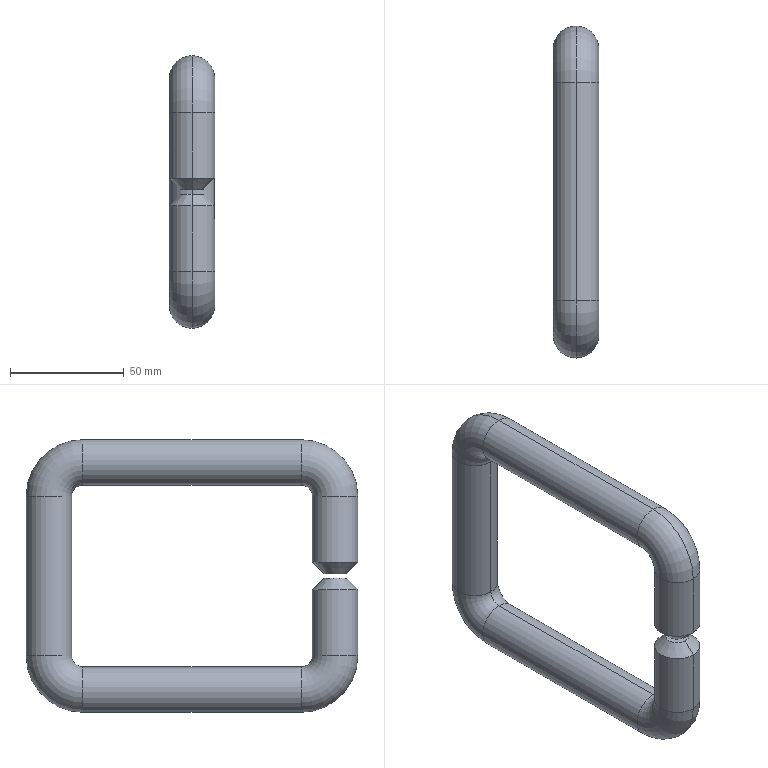Part | SolidWorks | features Chamfer 1, Sweep 1 | 1 solid | 24 faces | box 20 x 146 x 120 mm | volume 131972 mm3 | cylinder 10 | torus 8 | cone 4 | plane 2 | commonest cylinder face diameters 20 x10
STEP:
#1=CARTESIAN_POINT('',(0.,10.,34.));
#2=VERTEX_POINT('',#1);
#3=CARTESIAN_POINT('',(0.,-10.,34.));
#4=VERTEX_POINT('',#3);
#5=CARTESIAN_POINT('',(0.,0.,34.));
#6=DIRECTION('',(0.,0.,1.));
#7=DIRECTION('',(1.,0.,0.));
#8=AXIS2_PLACEMENT_3D('',#5,#6,#7);
#9=CIRCLE('',#8,10.);
#10=EDGE_CURVE('',#2,#4,#9,.T.);
#11=ORIENTED_EDGE('',*,*,#10,.T.);
#12=CARTESIAN_POINT('',(0.,15.,59.));
#13=VERTEX_POINT('',#12);
#14=CARTESIAN_POINT('',(0.,15.,34.));
#15=DIRECTION('',(-1.,0.,0.));
#16=DIRECTION('',(0.,0.,1.));
#17=AXIS2_PLACEMENT_3D('',#14,#15,#16);
#18=CIRCLE('',#17,25.);
#19=EDGE_CURVE('',#4,#13,#18,.T.);
#20=ORIENTED_EDGE('',*,*,#19,.T.);
#21=CARTESIAN_POINT('',(0.,15.,39.));
#22=VERTEX_POINT('',#21);
#23=CARTESIAN_POINT('',(0.,15.,49.));
#24=DIRECTION('',(0.,1.,0.));
#25=DIRECTION('',(1.,0.,0.));
#26=AXIS2_PLACEMENT_3D('',#23,#24,#25);
#27=CIRCLE('',#26,10.);
#28=EDGE_CURVE('',#22,#13,#27,.T.);
#29=ORIENTED_EDGE('',*,*,#28,.F.);
#30=CARTESIAN_POINT('',(0.,15.,34.));
#31=DIRECTION('',(-1.,0.,0.));
#32=DIRECTION('',(0.,0.,1.));
#33=AXIS2_PLACEMENT_3D('',#30,#31,#32);
#34=CIRCLE('',#33,5.);
#35=EDGE_CURVE('',#2,#22,#34,.T.);
#36=ORIENTED_EDGE('',*,*,#35,.F.);
#37=EDGE_LOOP('',(#11,#20,#29,#36));
#38=FACE_OUTER_BOUND('',#37,.T.);
#39=CARTESIAN_POINT('',(0.,15.,34.));
#40=DIRECTION('',(-1.,0.,0.));
#41=DIRECTION('',(0.,0.,1.));
#42=AXIS2_PLACEMENT_3D('',#39,#40,#41);
#43=TOROIDAL_SURFACE('',#42,15.,10.);
#44=ADVANCED_FACE('',(#38),#43,.T.);
#45=CARTESIAN_POINT('',(0.,111.,39.));
#46=VERTEX_POINT('',#45);
#47=CARTESIAN_POINT('',(0.,111.,59.));
#48=VERTEX_POINT('',#47);
#49=CARTESIAN_POINT('',(0.,111.,49.));
#50=DIRECTION('',(0.,1.,0.));
#51=DIRECTION('',(1.,0.,0.));
#52=AXIS2_PLACEMENT_3D('',#49,#50,#51);
#53=CIRCLE('',#52,10.);
#54=EDGE_CURVE('',#46,#48,#53,.T.);
#55=ORIENTED_EDGE('',*,*,#54,.T.);
#56=CARTESIAN_POINT('',(0.,136.,34.));
#57=VERTEX_POINT('',#56);
#58=CARTESIAN_POINT('',(0.,111.,34.));
#59=DIRECTION('',(-1.,0.,0.));
#60=DIRECTION('',(0.,0.,1.));
#61=AXIS2_PLACEMENT_3D('',#58,#59,#60);
#62=CIRCLE('',#61,25.);
#63=EDGE_CURVE('',#48,#57,#62,.T.);
#64=ORIENTED_EDGE('',*,*,#63,.T.);
#65=CARTESIAN_POINT('',(0.,116.,34.));
#66=VERTEX_POINT('',#65);
#67=CARTESIAN_POINT('',(0.,126.,34.));
#68=DIRECTION('',(0.,0.,-1.));
#69=DIRECTION('',(1.,0.,0.));
#70=AXIS2_PLACEMENT_3D('',#67,#68,#69);
#71=CIRCLE('',#70,10.);
#72=EDGE_CURVE('',#66,#57,#71,.T.);
#73=ORIENTED_EDGE('',*,*,#72,.F.);
#74=CARTESIAN_POINT('',(0.,111.,34.));
#75=DIRECTION('',(-1.,0.,0.));
#76=DIRECTION('',(0.,0.,1.));
#77=AXIS2_PLACEMENT_3D('',#74,#75,#76);
#78=CIRCLE('',#77,5.);
#79=EDGE_CURVE('',#46,#66,#78,.T.);
#80=ORIENTED_EDGE('',*,*,#79,.F.);
#81=EDGE_LOOP('',(#55,#64,#73,#80));
#82=FACE_OUTER_BOUND('',#81,.T.);
#83=CARTESIAN_POINT('',(0.,111.,34.));
#84=DIRECTION('',(-1.,0.,0.));
#85=DIRECTION('',(0.,0.,1.));
#86=AXIS2_PLACEMENT_3D('',#83,#84,#85);
#87=TOROIDAL_SURFACE('',#86,15.,10.);
#88=ADVANCED_FACE('',(#82),#87,.T.);
#89=CARTESIAN_POINT('',(0.,116.,-36.));
#90=VERTEX_POINT('',#89);
#91=CARTESIAN_POINT('',(0.,136.,-36.));
#92=VERTEX_POINT('',#91);
#93=CARTESIAN_POINT('',(0.,126.,-36.));
#94=DIRECTION('',(0.,0.,-1.));
#95=DIRECTION('',(1.,0.,0.));
#96=AXIS2_PLACEMENT_3D('',#93,#94,#95);
#97=CIRCLE('',#96,10.);
#98=EDGE_CURVE('',#90,#92,#97,.T.);
#99=ORIENTED_EDGE('',*,*,#98,.T.);
#100=CARTESIAN_POINT('',(0.,111.,-61.));
#101=VERTEX_POINT('',#100);
#102=CARTESIAN_POINT('',(0.,111.,-36.));
#103=DIRECTION('',(-1.,0.,0.));
#104=DIRECTION('',(0.,0.,1.));
#105=AXIS2_PLACEMENT_3D('',#102,#103,#104);
#106=CIRCLE('',#105,25.);
#107=EDGE_CURVE('',#92,#101,#106,.T.);
#108=ORIENTED_EDGE('',*,*,#107,.T.);
#109=CARTESIAN_POINT('',(0.,111.,-41.));
#110=VERTEX_POINT('',#109);
#111=CARTESIAN_POINT('',(0.,111.,-51.));
#112=DIRECTION('',(0.,-1.,0.));
#113=DIRECTION('',(1.,0.,0.));
#114=AXIS2_PLACEMENT_3D('',#111,#112,#113);
#115=CIRCLE('',#114,10.);
#116=EDGE_CURVE('',#110,#101,#115,.T.);
#117=ORIENTED_EDGE('',*,*,#116,.F.);
#118=CARTESIAN_POINT('',(0.,111.,-36.));
#119=DIRECTION('',(-1.,0.,0.));
#120=DIRECTION('',(0.,0.,1.));
#121=AXIS2_PLACEMENT_3D('',#118,#119,#120);
#122=CIRCLE('',#121,5.);
#123=EDGE_CURVE('',#90,#110,#122,.T.);
#124=ORIENTED_EDGE('',*,*,#123,.F.);
#125=EDGE_LOOP('',(#99,#108,#117,#124));
#126=FACE_OUTER_BOUND('',#125,.T.);
#127=CARTESIAN_POINT('',(0.,111.,-36.));
#128=DIRECTION('',(-1.,0.,0.));
#129=DIRECTION('',(0.,0.,1.));
#130=AXIS2_PLACEMENT_3D('',#127,#128,#129);
#131=TOROIDAL_SURFACE('',#130,15.,10.);
#132=ADVANCED_FACE('',(#126),#131,.T.);
#133=CARTESIAN_POINT('',(0.,15.,-41.));
#134=VERTEX_POINT('',#133);
#135=CARTESIAN_POINT('',(0.,15.,-61.));
#136=VERTEX_POINT('',#135);
#137=CARTESIAN_POINT('',(0.,15.,-51.));
#138=DIRECTION('',(0.,-1.,0.));
#139=DIRECTION('',(1.,0.,0.));
#140=AXIS2_PLACEMENT_3D('',#137,#138,#139);
#141=CIRCLE('',#140,10.);
#142=EDGE_CURVE('',#134,#136,#141,.T.);
#143=ORIENTED_EDGE('',*,*,#142,.T.);
#144=CARTESIAN_POINT('',(0.,-10.,-36.));
#145=VERTEX_POINT('',#144);
#146=CARTESIAN_POINT('',(0.,15.,-36.));
#147=DIRECTION('',(-1.,0.,0.));
#148=DIRECTION('',(0.,0.,1.));
#149=AXIS2_PLACEMENT_3D('',#146,#147,#148);
#150=CIRCLE('',#149,25.);
#151=EDGE_CURVE('',#136,#145,#150,.T.);
#152=ORIENTED_EDGE('',*,*,#151,.T.);
#153=CARTESIAN_POINT('',(0.,10.,-36.));
#154=VERTEX_POINT('',#153);
#155=CARTESIAN_POINT('',(0.,0.,-36.));
#156=DIRECTION('',(0.,0.,1.));
#157=DIRECTION('',(1.,0.,0.));
#158=AXIS2_PLACEMENT_3D('',#155,#156,#157);
#159=CIRCLE('',#158,10.);
#160=EDGE_CURVE('',#154,#145,#159,.T.);
#161=ORIENTED_EDGE('',*,*,#160,.F.);
#162=CARTESIAN_POINT('',(0.,15.,-36.));
#163=DIRECTION('',(-1.,0.,0.));
#164=DIRECTION('',(0.,0.,1.));
#165=AXIS2_PLACEMENT_3D('',#162,#163,#164);
#166=CIRCLE('',#165,5.);
#167=EDGE_CURVE('',#134,#154,#166,.T.);
#168=ORIENTED_EDGE('',*,*,#167,.F.);
#169=EDGE_LOOP('',(#143,#152,#161,#168));
#170=FACE_OUTER_BOUND('',#169,.T.);
#171=CARTESIAN_POINT('',(0.,15.,-36.));
#172=DIRECTION('',(-1.,0.,0.));
#173=DIRECTION('',(0.,0.,1.));
#174=AXIS2_PLACEMENT_3D('',#171,#172,#173);
#175=TOROIDAL_SURFACE('',#174,15.,10.);
#176=ADVANCED_FACE('',(#170),#175,.T.);
#177=CARTESIAN_POINT('',(0.,5.,0.));
#178=VERTEX_POINT('',#177);
#179=CARTESIAN_POINT('',(0.,-5.,0.));
#180=VERTEX_POINT('',#179);
#181=CARTESIAN_POINT('',(0.,0.,0.));
#182=DIRECTION('',(0.,0.,-1.));
#183=DIRECTION('',(1.,0.,0.));
#184=AXIS2_PLACEMENT_3D('',#181,#182,#183);
#185=CIRCLE('',#184,5.);
#186=EDGE_CURVE('',#178,#180,#185,.T.);
#187=ORIENTED_EDGE('',*,*,#186,.F.);
#188=CARTESIAN_POINT('',(0.,10.,5.));
#189=VERTEX_POINT('',#188);
#190=CARTESIAN_POINT('',(0.,10.,5.));
#191=DIRECTION('',(0.,0.7071,0.7071));
#192=VECTOR('',#191,1000.);
#193=LINE('',#190,#192);
#194=EDGE_CURVE('',#178,#189,#193,.T.);
#195=ORIENTED_EDGE('',*,*,#194,.T.);
#196=CARTESIAN_POINT('',(0.,-10.,5.));
#197=VERTEX_POINT('',#196);
#198=CARTESIAN_POINT('',(0.,0.,5.));
#199=DIRECTION('',(0.,0.,1.));
#200=DIRECTION('',(0.,-1.,0.));
#201=AXIS2_PLACEMENT_3D('',#198,#199,#200);
#202=CIRCLE('',#201,10.);
#203=EDGE_CURVE('',#197,#189,#202,.T.);
#204=ORIENTED_EDGE('',*,*,#203,.F.);
#205=CARTESIAN_POINT('',(0.,-10.,5.));
#206=DIRECTION('',(0.,-0.7071,0.7071));
#207=VECTOR('',#206,1000.);
#208=LINE('',#205,#207);
#209=EDGE_CURVE('',#180,#197,#208,.T.);
#210=ORIENTED_EDGE('',*,*,#209,.F.);
#211=EDGE_LOOP('',(#187,#195,#204,#210));
#212=FACE_OUTER_BOUND('',#211,.T.);
#213=CARTESIAN_POINT('',(0.,0.,5.));
#214=DIRECTION('',(0.,0.,1.));
#215=DIRECTION('',(0.,-1.,0.));
#216=AXIS2_PLACEMENT_3D('',#213,#214,#215);
#217=CONICAL_SURFACE('',#216,10.,0.7854);
#218=ADVANCED_FACE('',(#212),#217,.T.);
#219=CARTESIAN_POINT('',(0.,-5.,-2.));
#220=VERTEX_POINT('',#219);
#221=CARTESIAN_POINT('',(0.,5.,-2.));
#222=VERTEX_POINT('',#221);
#223=CARTESIAN_POINT('',(0.,0.,-2.));
#224=DIRECTION('',(0.,0.,1.));
#225=DIRECTION('',(0.,-1.,0.));
#226=AXIS2_PLACEMENT_3D('',#223,#224,#225);
#227=CIRCLE('',#226,5.);
#228=EDGE_CURVE('',#220,#222,#227,.T.);
#229=ORIENTED_EDGE('',*,*,#228,.F.);
#230=CARTESIAN_POINT('',(0.,-10.,-7.));
#231=VERTEX_POINT('',#230);
#232=CARTESIAN_POINT('',(0.,-5.,-2.));
#233=DIRECTION('',(0.,-0.7071,-0.7071));
#234=VECTOR('',#233,1000.);
#235=LINE('',#232,#234);
#236=EDGE_CURVE('',#220,#231,#235,.T.);
#237=ORIENTED_EDGE('',*,*,#236,.T.);
#238=CARTESIAN_POINT('',(0.,10.,-7.));
#239=VERTEX_POINT('',#238);
#240=CARTESIAN_POINT('',(0.,0.,-7.));
#241=DIRECTION('',(0.,0.,-1.));
#242=DIRECTION('',(0.,-1.,0.));
#243=AXIS2_PLACEMENT_3D('',#240,#241,#242);
#244=CIRCLE('',#243,10.);
#245=EDGE_CURVE('',#239,#231,#244,.T.);
#246=ORIENTED_EDGE('',*,*,#245,.F.);
#247=CARTESIAN_POINT('',(0.,5.,-2.));
#248=DIRECTION('',(0.,0.7071,-0.7071));
#249=VECTOR('',#248,1000.);
#250=LINE('',#247,#249);
#251=EDGE_CURVE('',#222,#239,#250,.T.);
#252=ORIENTED_EDGE('',*,*,#251,.F.);
#253=EDGE_LOOP('',(#229,#237,#246,#252));
#254=FACE_OUTER_BOUND('',#253,.T.);
#255=CARTESIAN_POINT('',(0.,0.,-2.));
#256=DIRECTION('',(0.,0.,-1.));
#257=DIRECTION('',(0.,1.,0.));
#258=AXIS2_PLACEMENT_3D('',#255,#256,#257);
#259=CONICAL_SURFACE('',#258,5.,0.7854);
#260=ADVANCED_FACE('',(#254),#259,.T.);
#261=CARTESIAN_POINT('',(0.,0.,34.));
#262=DIRECTION('',(0.,0.,1.));
#263=DIRECTION('',(1.,0.,0.));
#264=AXIS2_PLACEMENT_3D('',#261,#262,#263);
#265=CIRCLE('',#264,10.);
#266=EDGE_CURVE('',#4,#2,#265,.T.);
#267=ORIENTED_EDGE('',*,*,#266,.F.);
#268=CARTESIAN_POINT('',(0.,-10.,34.));
#269=DIRECTION('',(0.,0.,-1.));
#270=VECTOR('',#269,1000.);
#271=LINE('',#268,#270);
#272=EDGE_CURVE('',#4,#197,#271,.T.);
#273=ORIENTED_EDGE('',*,*,#272,.T.);
#274=ORIENTED_EDGE('',*,*,#203,.T.);
#275=CARTESIAN_POINT('',(0.,10.,34.));
#276=DIRECTION('',(0.,0.,-1.));
#277=VECTOR('',#276,1000.);
#278=LINE('',#275,#277);
#279=EDGE_CURVE('',#2,#189,#278,.T.);
#280=ORIENTED_EDGE('',*,*,#279,.F.);
#281=EDGE_LOOP('',(#267,#273,#274,#280));
#282=FACE_OUTER_BOUND('',#281,.T.);
#283=CARTESIAN_POINT('',(0.,0.,34.));
#284=DIRECTION('',(0.,0.,-1.));
#285=DIRECTION('',(0.,1.,0.));
#286=AXIS2_PLACEMENT_3D('',#283,#284,#285);
#287=CYLINDRICAL_SURFACE('',#286,10.);
#288=ADVANCED_FACE('',(#282),#287,.T.);
#289=CARTESIAN_POINT('',(0.,15.,49.));
#290=DIRECTION('',(0.,1.,0.));
#291=DIRECTION('',(1.,0.,0.));
#292=AXIS2_PLACEMENT_3D('',#289,#290,#291);
#293=CIRCLE('',#292,10.);
#294=EDGE_CURVE('',#13,#22,#293,.T.);
#295=ORIENTED_EDGE('',*,*,#294,.T.);
#296=CARTESIAN_POINT('',(0.,15.,39.));
#297=DIRECTION('',(0.,1.,0.));
#298=VECTOR('',#297,1000.);
#299=LINE('',#296,#298);
#300=EDGE_CURVE('',#22,#46,#299,.T.);
#301=ORIENTED_EDGE('',*,*,#300,.T.);
#302=CARTESIAN_POINT('',(0.,111.,49.));
#303=DIRECTION('',(0.,1.,0.));
#304=DIRECTION('',(1.,0.,0.));
#305=AXIS2_PLACEMENT_3D('',#302,#303,#304);
#306=CIRCLE('',#305,10.);
#307=EDGE_CURVE('',#48,#46,#306,.T.);
#308=ORIENTED_EDGE('',*,*,#307,.F.);
#309=CARTESIAN_POINT('',(0.,15.,59.));
#310=DIRECTION('',(0.,1.,0.));
#311=VECTOR('',#310,1000.);
#312=LINE('',#309,#311);
#313=EDGE_CURVE('',#13,#48,#312,.T.);
#314=ORIENTED_EDGE('',*,*,#313,.F.);
#315=EDGE_LOOP('',(#295,#301,#308,#314));
#316=FACE_OUTER_BOUND('',#315,.T.);
#317=CARTESIAN_POINT('',(0.,15.,49.));
#318=DIRECTION('',(0.,1.,0.));
#319=DIRECTION('',(0.,0.,1.));
#320=AXIS2_PLACEMENT_3D('',#317,#318,#319);
#321=CYLINDRICAL_SURFACE('',#320,10.);
#322=ADVANCED_FACE('',(#316),#321,.T.);
#323=CARTESIAN_POINT('',(0.,126.,34.));
#324=DIRECTION('',(0.,0.,-1.));
#325=DIRECTION('',(1.,0.,0.));
#326=AXIS2_PLACEMENT_3D('',#323,#324,#325);
#327=CIRCLE('',#326,10.);
#328=EDGE_CURVE('',#57,#66,#327,.T.);
#329=ORIENTED_EDGE('',*,*,#328,.T.);
#330=CARTESIAN_POINT('',(0.,116.,34.));
#331=DIRECTION('',(0.,0.,-1.));
#332=VECTOR('',#331,1000.);
#333=LINE('',#330,#332);
#334=EDGE_CURVE('',#66,#90,#333,.T.);
#335=ORIENTED_EDGE('',*,*,#334,.T.);
#336=CARTESIAN_POINT('',(0.,126.,-36.));
#337=DIRECTION('',(0.,0.,-1.));
#338=DIRECTION('',(1.,0.,0.));
#339=AXIS2_PLACEMENT_3D('',#336,#337,#338);
#340=CIRCLE('',#339,10.);
#341=EDGE_CURVE('',#92,#90,#340,.T.);
#342=ORIENTED_EDGE('',*,*,#341,.F.);
#343=CARTESIAN_POINT('',(0.,136.,34.));
#344=DIRECTION('',(0.,0.,-1.));
#345=VECTOR('',#344,1000.);
#346=LINE('',#343,#345);
#347=EDGE_CURVE('',#57,#92,#346,.T.);
#348=ORIENTED_EDGE('',*,*,#347,.F.);
#349=EDGE_LOOP('',(#329,#335,#342,#348));
#350=FACE_OUTER_BOUND('',#349,.T.);
#351=CARTESIAN_POINT('',(0.,126.,34.));
#352=DIRECTION('',(0.,0.,-1.));
#353=DIRECTION('',(0.,1.,0.));
#354=AXIS2_PLACEMENT_3D('',#351,#352,#353);
#355=CYLINDRICAL_SURFACE('',#354,10.);
#356=ADVANCED_FACE('',(#350),#355,.T.);
#357=CARTESIAN_POINT('',(0.,111.,-51.));
#358=DIRECTION('',(0.,-1.,0.));
#359=DIRECTION('',(1.,0.,0.));
#360=AXIS2_PLACEMENT_3D('',#357,#358,#359);
#361=CIRCLE('',#360,10.);
#362=EDGE_CURVE('',#101,#110,#361,.T.);
#363=ORIENTED_EDGE('',*,*,#362,.T.);
#364=CARTESIAN_POINT('',(0.,111.,-41.));
#365=DIRECTION('',(0.,-1.,0.));
#366=VECTOR('',#365,1000.);
#367=LINE('',#364,#366);
#368=EDGE_CURVE('',#110,#134,#367,.T.);
#369=ORIENTED_EDGE('',*,*,#368,.T.);
#370=CARTESIAN_POINT('',(0.,15.,-51.));
#371=DIRECTION('',(0.,-1.,0.));
#372=DIRECTION('',(1.,0.,0.));
#373=AXIS2_PLACEMENT_3D('',#370,#371,#372);
#374=CIRCLE('',#373,10.);
#375=EDGE_CURVE('',#136,#134,#374,.T.);
#376=ORIENTED_EDGE('',*,*,#375,.F.);
#377=CARTESIAN_POINT('',(0.,111.,-61.));
#378=DIRECTION('',(0.,-1.,0.));
#379=VECTOR('',#378,1000.);
#380=LINE('',#377,#379);
#381=EDGE_CURVE('',#101,#136,#380,.T.);
#382=ORIENTED_EDGE('',*,*,#381,.F.);
#383=EDGE_LOOP('',(#363,#369,#376,#382));
#384=FACE_OUTER_BOUND('',#383,.T.);
#385=CARTESIAN_POINT('',(0.,111.,-51.));
#386=DIRECTION('',(0.,-1.,0.));
#387=DIRECTION('',(0.,0.,-1.));
#388=AXIS2_PLACEMENT_3D('',#385,#386,#387);
#389=CYLINDRICAL_SURFACE('',#388,10.);
#390=ADVANCED_FACE('',(#384),#389,.T.);
#391=CARTESIAN_POINT('',(0.,0.,-36.));
#392=DIRECTION('',(0.,0.,1.));
#393=DIRECTION('',(1.,0.,0.));
#394=AXIS2_PLACEMENT_3D('',#391,#392,#393);
#395=CIRCLE('',#394,10.);
#396=EDGE_CURVE('',#145,#154,#395,.T.);
#397=ORIENTED_EDGE('',*,*,#396,.T.);
#398=CARTESIAN_POINT('',(0.,10.,-36.));
#399=DIRECTION('',(0.,0.,1.));
#400=VECTOR('',#399,1000.);
#401=LINE('',#398,#400);
#402=EDGE_CURVE('',#154,#239,#401,.T.);
#403=ORIENTED_EDGE('',*,*,#402,.T.);
#404=ORIENTED_EDGE('',*,*,#245,.T.);
#405=CARTESIAN_POINT('',(0.,-10.,-36.));
#406=DIRECTION('',(0.,0.,1.));
#407=VECTOR('',#406,1000.);
#408=LINE('',#405,#407);
#409=EDGE_CURVE('',#145,#231,#408,.T.);
#410=ORIENTED_EDGE('',*,*,#409,.F.);
#411=EDGE_LOOP('',(#397,#403,#404,#410));
#412=FACE_OUTER_BOUND('',#411,.T.);
#413=CARTESIAN_POINT('',(0.,0.,-36.));
#414=DIRECTION('',(0.,0.,1.));
#415=DIRECTION('',(0.,-1.,0.));
#416=AXIS2_PLACEMENT_3D('',#413,#414,#415);
#417=CYLINDRICAL_SURFACE('',#416,10.);
#418=ADVANCED_FACE('',(#412),#417,.T.);
#419=ORIENTED_EDGE('',*,*,#402,.F.);
#420=ORIENTED_EDGE('',*,*,#160,.T.);
#421=ORIENTED_EDGE('',*,*,#409,.T.);
#422=CARTESIAN_POINT('',(0.,0.,-7.));
#423=DIRECTION('',(0.,0.,-1.));
#424=DIRECTION('',(0.,-1.,0.));
#425=AXIS2_PLACEMENT_3D('',#422,#423,#424);
#426=CIRCLE('',#425,10.);
#427=EDGE_CURVE('',#231,#239,#426,.T.);
#428=ORIENTED_EDGE('',*,*,#427,.T.);
#429=EDGE_LOOP('',(#419,#420,#421,#428));
#430=FACE_OUTER_BOUND('',#429,.T.);
#431=CARTESIAN_POINT('',(0.,0.,-36.));
#432=DIRECTION('',(0.,0.,1.));
#433=DIRECTION('',(0.,-1.,0.));
#434=AXIS2_PLACEMENT_3D('',#431,#432,#433);
#435=CYLINDRICAL_SURFACE('',#434,10.);
#436=ADVANCED_FACE('',(#430),#435,.T.);
#437=ORIENTED_EDGE('',*,*,#151,.F.);
#438=ORIENTED_EDGE('',*,*,#375,.T.);
#439=ORIENTED_EDGE('',*,*,#167,.T.);
#440=ORIENTED_EDGE('',*,*,#396,.F.);
#441=EDGE_LOOP('',(#437,#438,#439,#440));
#442=FACE_OUTER_BOUND('',#441,.T.);
#443=CARTESIAN_POINT('',(0.,15.,-36.));
#444=DIRECTION('',(-1.,0.,0.));
#445=DIRECTION('',(0.,0.,1.));
#446=AXIS2_PLACEMENT_3D('',#443,#444,#445);
#447=TOROIDAL_SURFACE('',#446,15.,10.);
#448=ADVANCED_FACE('',(#442),#447,.T.);
#449=ORIENTED_EDGE('',*,*,#368,.F.);
#450=ORIENTED_EDGE('',*,*,#116,.T.);
#451=ORIENTED_EDGE('',*,*,#381,.T.);
#452=ORIENTED_EDGE('',*,*,#142,.F.);
#453=EDGE_LOOP('',(#449,#450,#451,#452));
#454=FACE_OUTER_BOUND('',#453,.T.);
#455=CARTESIAN_POINT('',(0.,111.,-51.));
#456=DIRECTION('',(0.,-1.,0.));
#457=DIRECTION('',(0.,0.,-1.));
#458=AXIS2_PLACEMENT_3D('',#455,#456,#457);
#459=CYLINDRICAL_SURFACE('',#458,10.);
#460=ADVANCED_FACE('',(#454),#459,.T.);
#461=ORIENTED_EDGE('',*,*,#107,.F.);
#462=ORIENTED_EDGE('',*,*,#341,.T.);
#463=ORIENTED_EDGE('',*,*,#123,.T.);
#464=ORIENTED_EDGE('',*,*,#362,.F.);
#465=EDGE_LOOP('',(#461,#462,#463,#464));
#466=FACE_OUTER_BOUND('',#465,.T.);
#467=CARTESIAN_POINT('',(0.,111.,-36.));
#468=DIRECTION('',(-1.,0.,0.));
#469=DIRECTION('',(0.,0.,1.));
#470=AXIS2_PLACEMENT_3D('',#467,#468,#469);
#471=TOROIDAL_SURFACE('',#470,15.,10.);
#472=ADVANCED_FACE('',(#466),#471,.T.);
#473=ORIENTED_EDGE('',*,*,#334,.F.);
#474=ORIENTED_EDGE('',*,*,#72,.T.);
#475=ORIENTED_EDGE('',*,*,#347,.T.);
#476=ORIENTED_EDGE('',*,*,#98,.F.);
#477=EDGE_LOOP('',(#473,#474,#475,#476));
#478=FACE_OUTER_BOUND('',#477,.T.);
#479=CARTESIAN_POINT('',(0.,126.,34.));
#480=DIRECTION('',(0.,0.,-1.));
#481=DIRECTION('',(0.,1.,0.));
#482=AXIS2_PLACEMENT_3D('',#479,#480,#481);
#483=CYLINDRICAL_SURFACE('',#482,10.);
#484=ADVANCED_FACE('',(#478),#483,.T.);
#485=ORIENTED_EDGE('',*,*,#63,.F.);
#486=ORIENTED_EDGE('',*,*,#307,.T.);
#487=ORIENTED_EDGE('',*,*,#79,.T.);
#488=ORIENTED_EDGE('',*,*,#328,.F.);
#489=EDGE_LOOP('',(#485,#486,#487,#488));
#490=FACE_OUTER_BOUND('',#489,.T.);
#491=CARTESIAN_POINT('',(0.,111.,34.));
#492=DIRECTION('',(-1.,0.,0.));
#493=DIRECTION('',(0.,0.,1.));
#494=AXIS2_PLACEMENT_3D('',#491,#492,#493);
#495=TOROIDAL_SURFACE('',#494,15.,10.);
#496=ADVANCED_FACE('',(#490),#495,.T.);
#497=ORIENTED_EDGE('',*,*,#300,.F.);
#498=ORIENTED_EDGE('',*,*,#28,.T.);
#499=ORIENTED_EDGE('',*,*,#313,.T.);
#500=ORIENTED_EDGE('',*,*,#54,.F.);
#501=EDGE_LOOP('',(#497,#498,#499,#500));
#502=FACE_OUTER_BOUND('',#501,.T.);
#503=CARTESIAN_POINT('',(0.,15.,49.));
#504=DIRECTION('',(0.,1.,0.));
#505=DIRECTION('',(0.,0.,1.));
#506=AXIS2_PLACEMENT_3D('',#503,#504,#505);
#507=CYLINDRICAL_SURFACE('',#506,10.);
#508=ADVANCED_FACE('',(#502),#507,.T.);
#509=ORIENTED_EDGE('',*,*,#19,.F.);
#510=ORIENTED_EDGE('',*,*,#266,.T.);
#511=ORIENTED_EDGE('',*,*,#35,.T.);
#512=ORIENTED_EDGE('',*,*,#294,.F.);
#513=EDGE_LOOP('',(#509,#510,#511,#512));
#514=FACE_OUTER_BOUND('',#513,.T.);
#515=CARTESIAN_POINT('',(0.,15.,34.));
#516=DIRECTION('',(-1.,0.,0.));
#517=DIRECTION('',(0.,0.,1.));
#518=AXIS2_PLACEMENT_3D('',#515,#516,#517);
#519=TOROIDAL_SURFACE('',#518,15.,10.);
#520=ADVANCED_FACE('',(#514),#519,.T.);
#521=ORIENTED_EDGE('',*,*,#272,.F.);
#522=ORIENTED_EDGE('',*,*,#10,.F.);
#523=ORIENTED_EDGE('',*,*,#279,.T.);
#524=CARTESIAN_POINT('',(0.,0.,5.));
#525=DIRECTION('',(0.,0.,1.));
#526=DIRECTION('',(0.,-1.,0.));
#527=AXIS2_PLACEMENT_3D('',#524,#525,#526);
#528=CIRCLE('',#527,10.);
#529=EDGE_CURVE('',#189,#197,#528,.T.);
#530=ORIENTED_EDGE('',*,*,#529,.T.);
#531=EDGE_LOOP('',(#521,#522,#523,#530));
#532=FACE_OUTER_BOUND('',#531,.T.);
#533=CARTESIAN_POINT('',(0.,0.,34.));
#534=DIRECTION('',(0.,0.,-1.));
#535=DIRECTION('',(0.,1.,0.));
#536=AXIS2_PLACEMENT_3D('',#533,#534,#535);
#537=CYLINDRICAL_SURFACE('',#536,10.);
#538=ADVANCED_FACE('',(#532),#537,.T.);
#539=CARTESIAN_POINT('',(0.,0.,-2.));
#540=DIRECTION('',(0.,0.,1.));
#541=DIRECTION('',(0.,-1.,0.));
#542=AXIS2_PLACEMENT_3D('',#539,#540,#541);
#543=CIRCLE('',#542,5.);
#544=EDGE_CURVE('',#222,#220,#543,.T.);
#545=ORIENTED_EDGE('',*,*,#544,.T.);
#546=ORIENTED_EDGE('',*,*,#228,.T.);
#547=EDGE_LOOP('',(#545,#546));
#548=FACE_OUTER_BOUND('',#547,.T.);
#549=CARTESIAN_POINT('',(0.,0.,-2.));
#550=DIRECTION('',(0.,0.,1.));
#551=DIRECTION('',(1.,0.,0.));
#552=AXIS2_PLACEMENT_3D('',#549,#550,#551);
#553=PLANE('',#552);
#554=ADVANCED_FACE('',(#548),#553,.T.);
#555=CARTESIAN_POINT('',(0.,0.,0.));
#556=DIRECTION('',(0.,0.,-1.));
#557=DIRECTION('',(1.,0.,0.));
#558=AXIS2_PLACEMENT_3D('',#555,#556,#557);
#559=CIRCLE('',#558,5.);
#560=EDGE_CURVE('',#180,#178,#559,.T.);
#561=ORIENTED_EDGE('',*,*,#560,.T.);
#562=ORIENTED_EDGE('',*,*,#186,.T.);
#563=EDGE_LOOP('',(#561,#562));
#564=FACE_OUTER_BOUND('',#563,.T.);
#565=CARTESIAN_POINT('',(0.,0.,0.));
#566=DIRECTION('',(0.,0.,1.));
#567=DIRECTION('',(1.,0.,0.));
#568=AXIS2_PLACEMENT_3D('',#565,#566,#567);
#569=PLANE('',#568);
#570=ADVANCED_FACE('',(#564),#569,.F.);
#571=ORIENTED_EDGE('',*,*,#236,.F.);
#572=ORIENTED_EDGE('',*,*,#544,.F.);
#573=ORIENTED_EDGE('',*,*,#251,.T.);
#574=ORIENTED_EDGE('',*,*,#427,.F.);
#575=EDGE_LOOP('',(#571,#572,#573,#574));
#576=FACE_OUTER_BOUND('',#575,.T.);
#577=CARTESIAN_POINT('',(0.,0.,-2.));
#578=DIRECTION('',(0.,0.,-1.));
#579=DIRECTION('',(0.,1.,0.));
#580=AXIS2_PLACEMENT_3D('',#577,#578,#579);
#581=CONICAL_SURFACE('',#580,5.,0.7854);
#582=ADVANCED_FACE('',(#576),#581,.T.);
#583=ORIENTED_EDGE('',*,*,#194,.F.);
#584=ORIENTED_EDGE('',*,*,#560,.F.);
#585=ORIENTED_EDGE('',*,*,#209,.T.);
#586=ORIENTED_EDGE('',*,*,#529,.F.);
#587=EDGE_LOOP('',(#583,#584,#585,#586));
#588=FACE_OUTER_BOUND('',#587,.T.);
#589=CARTESIAN_POINT('',(0.,0.,5.));
#590=DIRECTION('',(0.,0.,1.));
#591=DIRECTION('',(0.,-1.,0.));
#592=AXIS2_PLACEMENT_3D('',#589,#590,#591);
#593=CONICAL_SURFACE('',#592,10.,0.7854);
#594=ADVANCED_FACE('',(#588),#593,.T.);
#595=CLOSED_SHELL('',(#44,#88,#132,#176,#218,#260,#288,#322,#356,#390,#418,#436,#448,#460,#472,#484,#496,#508,#520,#538,#554,#570,#582,#594));
#596=MANIFOLD_SOLID_BREP('',#595);
#597=CARTESIAN_POINT('',(0.,0.,0.));
#598=DIRECTION('',(0.,0.,1.));
#599=DIRECTION('',(1.,0.,0.));
#600=AXIS2_PLACEMENT_3D('',#597,#598,#599);
#601=(LENGTH_UNIT()NAMED_UNIT(*)SI_UNIT(.MILLI.,.METRE.));
#602=UNCERTAINTY_MEASURE_WITH_UNIT(LENGTH_MEASURE(0.00001),#601,'','');
#603=(NAMED_UNIT(*)PLANE_ANGLE_UNIT()SI_UNIT($,.RADIAN.));
#604=(NAMED_UNIT(*)SI_UNIT($,.STERADIAN.)SOLID_ANGLE_UNIT());
#605=(GEOMETRIC_REPRESENTATION_CONTEXT(3)GLOBAL_UNCERTAINTY_ASSIGNED_CONTEXT((#602))GLOBAL_UNIT_ASSIGNED_CONTEXT((#601,#603,#604))REPRESENTATION_CONTEXT('',''));
#606=ADVANCED_BREP_SHAPE_REPRESENTATION('',(#596,#600),#605);